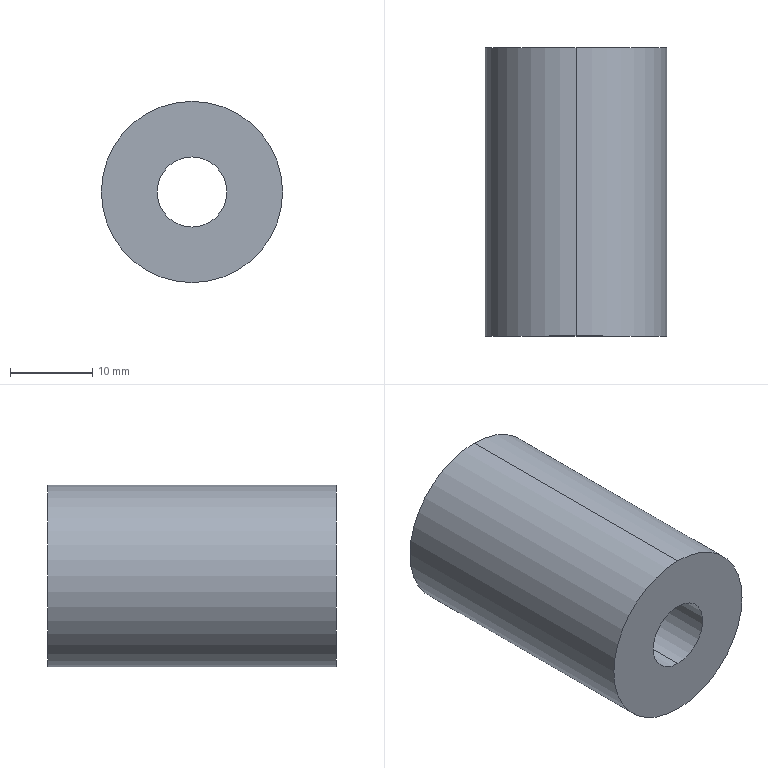Part | SolidWorks | features Extrusion 1, HoleWzd 1 | 1 solid | 6 faces | box 22 x 35 x 22 mm | volume 11319 mm3 | cylinder 4 | plane 2 | commonest cylinder face diameters 8.5 x2 22 x2
STEP:
#1=CARTESIAN_POINT('',(0.,0.,-4.25));
#2=VERTEX_POINT('',#1);
#3=CARTESIAN_POINT('',(0.,0.,4.25));
#4=VERTEX_POINT('',#3);
#5=CARTESIAN_POINT('',(0.,0.,0.));
#6=DIRECTION('',(0.,1.,0.));
#7=DIRECTION('',(0.,0.,1.));
#8=AXIS2_PLACEMENT_3D('',#5,#6,#7);
#9=CIRCLE('',#8,4.25);
#10=EDGE_CURVE('',#2,#4,#9,.T.);
#11=ORIENTED_EDGE('',*,*,#10,.F.);
#12=CARTESIAN_POINT('',(0.,35.,-4.25));
#13=VERTEX_POINT('',#12);
#14=CARTESIAN_POINT('',(0.,35.,-4.25));
#15=DIRECTION('',(0.,1.,0.));
#16=VECTOR('',#15,1000.);
#17=LINE('',#14,#16);
#18=EDGE_CURVE('',#2,#13,#17,.T.);
#19=ORIENTED_EDGE('',*,*,#18,.T.);
#20=CARTESIAN_POINT('',(0.,35.,4.25));
#21=VERTEX_POINT('',#20);
#22=CARTESIAN_POINT('',(0.,35.,0.));
#23=DIRECTION('',(0.,1.,0.));
#24=DIRECTION('',(0.,0.,1.));
#25=AXIS2_PLACEMENT_3D('',#22,#23,#24);
#26=CIRCLE('',#25,4.25);
#27=EDGE_CURVE('',#13,#21,#26,.T.);
#28=ORIENTED_EDGE('',*,*,#27,.T.);
#29=CARTESIAN_POINT('',(0.,35.,4.25));
#30=DIRECTION('',(0.,1.,0.));
#31=VECTOR('',#30,1000.);
#32=LINE('',#29,#31);
#33=EDGE_CURVE('',#4,#21,#32,.T.);
#34=ORIENTED_EDGE('',*,*,#33,.F.);
#35=EDGE_LOOP('',(#11,#19,#28,#34));
#36=FACE_OUTER_BOUND('',#35,.T.);
#37=CARTESIAN_POINT('',(0.,35.,0.));
#38=DIRECTION('',(0.,1.,0.));
#39=DIRECTION('',(0.,0.,1.));
#40=AXIS2_PLACEMENT_3D('',#37,#38,#39);
#41=CYLINDRICAL_SURFACE('',#40,4.25);
#42=ADVANCED_FACE('',(#36),#41,.F.);
#43=CARTESIAN_POINT('',(0.,35.,11.));
#44=VERTEX_POINT('',#43);
#45=CARTESIAN_POINT('',(0.,35.,-11.));
#46=VERTEX_POINT('',#45);
#47=CARTESIAN_POINT('',(0.,35.,0.));
#48=DIRECTION('',(0.,1.,0.));
#49=DIRECTION('',(0.,0.,1.));
#50=AXIS2_PLACEMENT_3D('',#47,#48,#49);
#51=CIRCLE('',#50,11.);
#52=EDGE_CURVE('',#44,#46,#51,.T.);
#53=ORIENTED_EDGE('',*,*,#52,.F.);
#54=CARTESIAN_POINT('',(0.,0.,11.));
#55=VERTEX_POINT('',#54);
#56=CARTESIAN_POINT('',(0.,35.,11.));
#57=DIRECTION('',(0.,-1.,0.));
#58=VECTOR('',#57,1000.);
#59=LINE('',#56,#58);
#60=EDGE_CURVE('',#44,#55,#59,.T.);
#61=ORIENTED_EDGE('',*,*,#60,.T.);
#62=CARTESIAN_POINT('',(0.,0.,-11.));
#63=VERTEX_POINT('',#62);
#64=CARTESIAN_POINT('',(0.,0.,0.));
#65=DIRECTION('',(0.,1.,0.));
#66=DIRECTION('',(0.,0.,1.));
#67=AXIS2_PLACEMENT_3D('',#64,#65,#66);
#68=CIRCLE('',#67,11.);
#69=EDGE_CURVE('',#55,#63,#68,.T.);
#70=ORIENTED_EDGE('',*,*,#69,.T.);
#71=CARTESIAN_POINT('',(0.,35.,-11.));
#72=DIRECTION('',(0.,-1.,0.));
#73=VECTOR('',#72,1000.);
#74=LINE('',#71,#73);
#75=EDGE_CURVE('',#46,#63,#74,.T.);
#76=ORIENTED_EDGE('',*,*,#75,.F.);
#77=EDGE_LOOP('',(#53,#61,#70,#76));
#78=FACE_OUTER_BOUND('',#77,.T.);
#79=CARTESIAN_POINT('',(0.,35.,0.));
#80=DIRECTION('',(0.,-1.,0.));
#81=DIRECTION('',(0.,0.,-1.));
#82=AXIS2_PLACEMENT_3D('',#79,#80,#81);
#83=CYLINDRICAL_SURFACE('',#82,11.);
#84=ADVANCED_FACE('',(#78),#83,.T.);
#85=ORIENTED_EDGE('',*,*,#60,.F.);
#86=CARTESIAN_POINT('',(0.,35.,0.));
#87=DIRECTION('',(0.,1.,0.));
#88=DIRECTION('',(0.,0.,1.));
#89=AXIS2_PLACEMENT_3D('',#86,#87,#88);
#90=CIRCLE('',#89,11.);
#91=EDGE_CURVE('',#46,#44,#90,.T.);
#92=ORIENTED_EDGE('',*,*,#91,.F.);
#93=ORIENTED_EDGE('',*,*,#75,.T.);
#94=CARTESIAN_POINT('',(0.,0.,0.));
#95=DIRECTION('',(0.,1.,0.));
#96=DIRECTION('',(0.,0.,1.));
#97=AXIS2_PLACEMENT_3D('',#94,#95,#96);
#98=CIRCLE('',#97,11.);
#99=EDGE_CURVE('',#63,#55,#98,.T.);
#100=ORIENTED_EDGE('',*,*,#99,.T.);
#101=EDGE_LOOP('',(#85,#92,#93,#100));
#102=FACE_OUTER_BOUND('',#101,.T.);
#103=CARTESIAN_POINT('',(0.,35.,0.));
#104=DIRECTION('',(0.,-1.,0.));
#105=DIRECTION('',(0.,0.,-1.));
#106=AXIS2_PLACEMENT_3D('',#103,#104,#105);
#107=CYLINDRICAL_SURFACE('',#106,11.);
#108=ADVANCED_FACE('',(#102),#107,.T.);
#109=CARTESIAN_POINT('',(0.,35.,0.));
#110=DIRECTION('',(0.,1.,0.));
#111=DIRECTION('',(0.,0.,1.));
#112=AXIS2_PLACEMENT_3D('',#109,#110,#111);
#113=CIRCLE('',#112,4.25);
#114=EDGE_CURVE('',#21,#13,#113,.T.);
#115=ORIENTED_EDGE('',*,*,#114,.F.);
#116=ORIENTED_EDGE('',*,*,#27,.F.);
#117=EDGE_LOOP('',(#115,#116));
#118=FACE_BOUND('',#117,.T.);
#119=ORIENTED_EDGE('',*,*,#91,.T.);
#120=ORIENTED_EDGE('',*,*,#52,.T.);
#121=EDGE_LOOP('',(#119,#120));
#122=FACE_OUTER_BOUND('',#121,.T.);
#123=CARTESIAN_POINT('',(0.,35.,0.));
#124=DIRECTION('',(0.,1.,0.));
#125=DIRECTION('',(0.,0.,1.));
#126=AXIS2_PLACEMENT_3D('',#123,#124,#125);
#127=PLANE('',#126);
#128=ADVANCED_FACE('',(#118,#122),#127,.T.);
#129=CARTESIAN_POINT('',(0.,0.,0.));
#130=DIRECTION('',(0.,1.,0.));
#131=DIRECTION('',(0.,0.,1.));
#132=AXIS2_PLACEMENT_3D('',#129,#130,#131);
#133=CIRCLE('',#132,4.25);
#134=EDGE_CURVE('',#4,#2,#133,.T.);
#135=ORIENTED_EDGE('',*,*,#134,.T.);
#136=ORIENTED_EDGE('',*,*,#10,.T.);
#137=EDGE_LOOP('',(#135,#136));
#138=FACE_BOUND('',#137,.T.);
#139=ORIENTED_EDGE('',*,*,#99,.F.);
#140=ORIENTED_EDGE('',*,*,#69,.F.);
#141=EDGE_LOOP('',(#139,#140));
#142=FACE_OUTER_BOUND('',#141,.T.);
#143=CARTESIAN_POINT('',(0.,0.,0.));
#144=DIRECTION('',(0.,1.,0.));
#145=DIRECTION('',(0.,0.,1.));
#146=AXIS2_PLACEMENT_3D('',#143,#144,#145);
#147=PLANE('',#146);
#148=ADVANCED_FACE('',(#138,#142),#147,.F.);
#149=ORIENTED_EDGE('',*,*,#18,.F.);
#150=ORIENTED_EDGE('',*,*,#134,.F.);
#151=ORIENTED_EDGE('',*,*,#33,.T.);
#152=ORIENTED_EDGE('',*,*,#114,.T.);
#153=EDGE_LOOP('',(#149,#150,#151,#152));
#154=FACE_OUTER_BOUND('',#153,.T.);
#155=CARTESIAN_POINT('',(0.,35.,0.));
#156=DIRECTION('',(0.,1.,0.));
#157=DIRECTION('',(0.,0.,1.));
#158=AXIS2_PLACEMENT_3D('',#155,#156,#157);
#159=CYLINDRICAL_SURFACE('',#158,4.25);
#160=ADVANCED_FACE('',(#154),#159,.F.);
#161=CLOSED_SHELL('',(#42,#84,#108,#128,#148,#160));
#162=MANIFOLD_SOLID_BREP('',#161);
#163=CARTESIAN_POINT('',(0.,0.,0.));
#164=DIRECTION('',(0.,0.,1.));
#165=DIRECTION('',(1.,0.,0.));
#166=AXIS2_PLACEMENT_3D('',#163,#164,#165);
#167=(LENGTH_UNIT()NAMED_UNIT(*)SI_UNIT(.MILLI.,.METRE.));
#168=UNCERTAINTY_MEASURE_WITH_UNIT(LENGTH_MEASURE(0.00001),#167,'','');
#169=(NAMED_UNIT(*)PLANE_ANGLE_UNIT()SI_UNIT($,.RADIAN.));
#170=(NAMED_UNIT(*)SI_UNIT($,.STERADIAN.)SOLID_ANGLE_UNIT());
#171=(GEOMETRIC_REPRESENTATION_CONTEXT(3)GLOBAL_UNCERTAINTY_ASSIGNED_CONTEXT((#168))GLOBAL_UNIT_ASSIGNED_CONTEXT((#167,#169,#170))REPRESENTATION_CONTEXT('',''));
#172=ADVANCED_BREP_SHAPE_REPRESENTATION('',(#162,#166),#171);